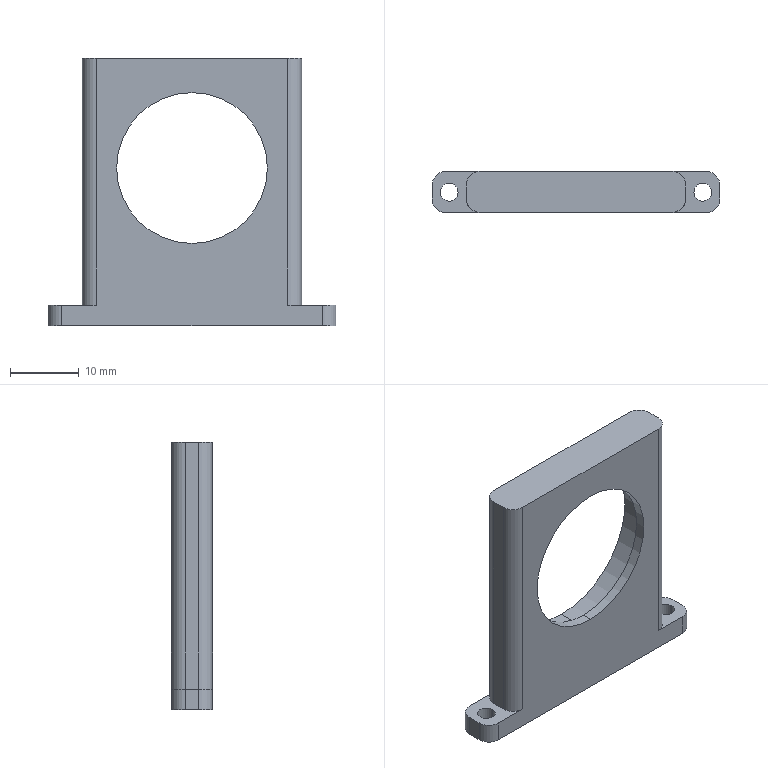NC program | NX | posted with a generic post | part box 42 x 6 x 39 mm
Whole program:
N10 G17 G21 G94 G90
(FLOOR_WALL_COPY_COPY , TOOL : D10JING)
N12 T14 M6
N14 G54
N16 G17 G0 G90 X-31. Y0. B0. C0. S6500 M3
N18 G43 Z30. H14
N20 Z8.
N22 G94 G1 Z5. F1500.
N24 X-26.
N26 X26.
N28 X31.
N30 Z8.
N32 G0 Z30.
N34 X-31.
N36 Z7.
N38 G1 Z4.
N40 X-26.
N42 X26.
N44 X31.
N46 Z7.
N48 G0 Z30.
N50 X-31.
N52 Z6.
N54 G1 Z3.
N56 X-26.
N58 X26.
N60 X31.
N62 Z6.
N64 G0 Z30.
N66 X-31.
N68 Z5.
N70 G1 Z2.
N72 X-26.
N74 X26.
N76 X31.
N78 Z5.
N80 G0 Z30.
N82 X-31.
N84 Z4.
N86 G1 Z1.
N88 X-26.
N90 X26.
N92 X31.
N94 Z4.
N96 G0 Z30.
N98 X-31.
N100 Z3.
N102 G1 Z0.
N104 X-26.
N106 X26.
N108 X31.
N110 Z3.
N112 G0 Z30.
N114 M5
(DRILLING_COPY_1_COPY , TOOL : D6A45)
N116 T01 M6
N118 G54
N120 G17 G0 G90 X0. Y0. B0. C0. S5000 M3
N122 G43 Z30. H1
N124 G94 G81 G98 Z-1. F350. R3.
N126 X18.5
N128 X-18.5
N130 G80
N132 G0 X-18.5 Y0. Z30.
N134 M5
(DRILLING_COPY_1_COPY_1_1_COPY_1 , TOOL : 3.3ZT)
N136 T03 M6
N138 G54
N140 G17 G0 G90 X0. Y0. B0. C0. S2000 M3
N142 G43 Z30. H3
N144 G94 G83 G98 Z-8. F200. Q2. R3.
N146 G80
N148 G0 X0. Y0. Z30.
N150 M5
(DRILLING_COPY_1_COPY_1_1_COPY_1_COPY , TOOL : 2.6ZT)
N152 T17 M6
N154 G54
N156 G17 G0 G90 X-18.5 Y0. B0. C0. S2000 M3
N158 G43 Z30. H17
N160 G94 G83 G98 Z-5.281 F200. Q2. R3.
N162 X18.5
N164 G80
N166 G0 X18.5 Y0. Z30.
N168 M5
(PLANAR_MILL_COPY_COPY_COPY_COPY_COPY_COPY_1_COPY_1_COPY , TOOL : D6A45)
N170 T01 M6
N172 G54
N174 G17 G0 G90 X18.75 Y-0.433 B0. C0. S9500 M3
N176 G43 Z30. H1
N178 Z0.5
N180 G94 G1 Z-1. F1250.
N182 G3 X19. Y0. R0.5
N184 X18.5 Y0.5 R0.5
N186 X19. Y0. R-0.5
N188 X18.75 Y0.433 R0.5
N190 G1 Z0.5
N192 G0 Z30.
N194 X0.433 Y0.6
N196 Z0.5
N198 G1 Z-1.
N200 G3 X0. Y0.85 R0.5
N202 X-0.85 Y0. R0.85
N204 X0. Y0.85 R-0.85
N206 X-0.433 Y0.6 R0.5
N208 G1 Z0.5
N210 G0 Z30.
N212 X0.866 Y-4.3
N214 Z0.5
N216 G1 Z-1.
N218 G3 X0. Y-3.8 R1.
N220 G1 X-19.
N222 G2 X-21.8 Y-1. R2.8
N224 G1 Y1.
N226 G2 X-19. Y3.8 R2.8
N228 G1 X19.
N230 G2 X21.8 Y1. R2.8
N232 G1 Y-1.
N234 G2 X19. Y-3.8 R2.8
N236 G1 X0.
N238 G3 X-0.866 Y-4.3 R1.
N240 G1 Z0.5
N242 G0 Z30.
N244 X-18.75 Y0.433
N246 Z0.5
N248 G1 Z-1.
N250 G3 X-19. Y0. R0.5
N252 X-18.5 Y-0.5 R0.5
N254 X-19. Y0. R-0.5
N256 X-18.75 Y-0.433 R0.5
N258 G1 Z0.5
N260 G0 Z30.
N262 M5
N264 M2